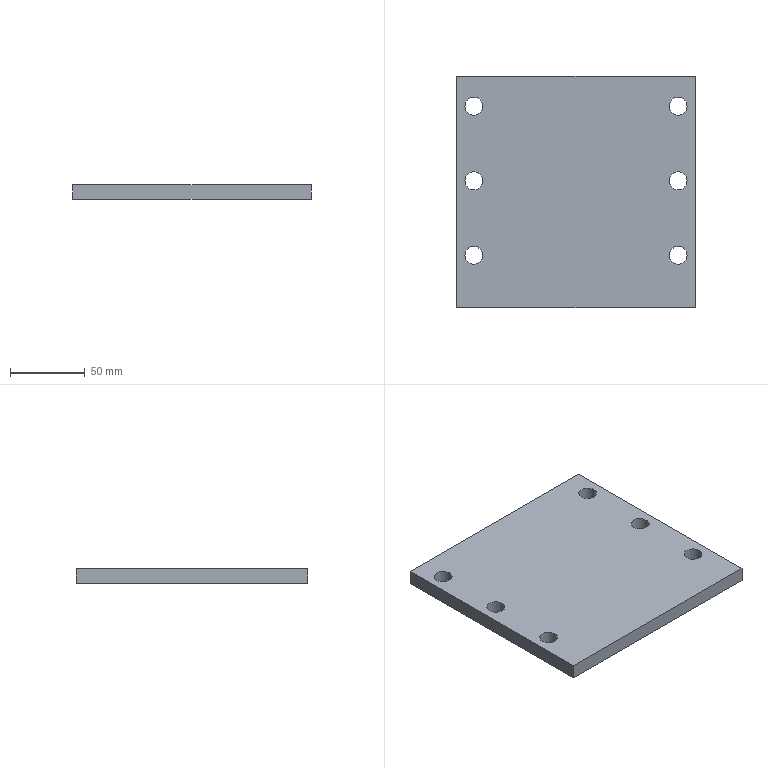Part | SolidWorks | features BaseBody 1 | 1 solid | 18 faces | box 160 x 155 x 10 mm | volume 241214 mm3 | cylinder 12 | plane 6 | commonest cylinder face diameters 12 x12
STEP:
#1=CARTESIAN_POINT('',(-0.01949,144.091,0.));
#2=VERTEX_POINT('',#1);
#3=CARTESIAN_POINT('',(-12.019,144.091,0.));
#4=VERTEX_POINT('',#3);
#5=CARTESIAN_POINT('',(-6.019,144.091,0.));
#6=DIRECTION('',(0.,0.,-1.));
#7=DIRECTION('',(1.,0.,0.));
#8=AXIS2_PLACEMENT_3D('',#5,#6,#7);
#9=CIRCLE('',#8,6.);
#10=EDGE_CURVE('',#2,#4,#9,.T.);
#11=ORIENTED_EDGE('',*,*,#10,.T.);
#12=CARTESIAN_POINT('',(-12.019,144.091,10.));
#13=VERTEX_POINT('',#12);
#14=CARTESIAN_POINT('',(-12.019,144.091,0.));
#15=DIRECTION('',(0.,0.,1.));
#16=VECTOR('',#15,1000.);
#17=LINE('',#14,#16);
#18=EDGE_CURVE('',#4,#13,#17,.T.);
#19=ORIENTED_EDGE('',*,*,#18,.T.);
#20=CARTESIAN_POINT('',(-0.01949,144.091,10.));
#21=VERTEX_POINT('',#20);
#22=CARTESIAN_POINT('',(-6.019,144.091,10.));
#23=DIRECTION('',(0.,0.,-1.));
#24=DIRECTION('',(1.,0.,0.));
#25=AXIS2_PLACEMENT_3D('',#22,#23,#24);
#26=CIRCLE('',#25,6.);
#27=EDGE_CURVE('',#21,#13,#26,.T.);
#28=ORIENTED_EDGE('',*,*,#27,.F.);
#29=CARTESIAN_POINT('',(-0.01949,144.091,0.));
#30=DIRECTION('',(0.,0.,1.));
#31=VECTOR('',#30,1000.);
#32=LINE('',#29,#31);
#33=EDGE_CURVE('',#2,#21,#32,.T.);
#34=ORIENTED_EDGE('',*,*,#33,.F.);
#35=EDGE_LOOP('',(#11,#19,#28,#34));
#36=FACE_OUTER_BOUND('',#35,.T.);
#37=CARTESIAN_POINT('',(-6.019,144.091,0.));
#38=DIRECTION('',(0.,0.,1.));
#39=DIRECTION('',(1.,0.,0.));
#40=AXIS2_PLACEMENT_3D('',#37,#38,#39);
#41=CYLINDRICAL_SURFACE('',#40,6.);
#42=ADVANCED_FACE('',(#36),#41,.F.);
#43=CARTESIAN_POINT('',(136.981,144.091,0.));
#44=VERTEX_POINT('',#43);
#45=CARTESIAN_POINT('',(124.981,144.091,0.));
#46=VERTEX_POINT('',#45);
#47=CARTESIAN_POINT('',(130.981,144.091,0.));
#48=DIRECTION('',(0.,0.,-1.));
#49=DIRECTION('',(1.,0.,0.));
#50=AXIS2_PLACEMENT_3D('',#47,#48,#49);
#51=CIRCLE('',#50,6.);
#52=EDGE_CURVE('',#44,#46,#51,.T.);
#53=ORIENTED_EDGE('',*,*,#52,.T.);
#54=CARTESIAN_POINT('',(124.981,144.091,10.));
#55=VERTEX_POINT('',#54);
#56=CARTESIAN_POINT('',(124.981,144.091,0.));
#57=DIRECTION('',(0.,0.,1.));
#58=VECTOR('',#57,1000.);
#59=LINE('',#56,#58);
#60=EDGE_CURVE('',#46,#55,#59,.T.);
#61=ORIENTED_EDGE('',*,*,#60,.T.);
#62=CARTESIAN_POINT('',(136.981,144.091,10.));
#63=VERTEX_POINT('',#62);
#64=CARTESIAN_POINT('',(130.981,144.091,10.));
#65=DIRECTION('',(0.,0.,-1.));
#66=DIRECTION('',(1.,0.,0.));
#67=AXIS2_PLACEMENT_3D('',#64,#65,#66);
#68=CIRCLE('',#67,6.);
#69=EDGE_CURVE('',#63,#55,#68,.T.);
#70=ORIENTED_EDGE('',*,*,#69,.F.);
#71=CARTESIAN_POINT('',(136.981,144.091,0.));
#72=DIRECTION('',(0.,0.,1.));
#73=VECTOR('',#72,1000.);
#74=LINE('',#71,#73);
#75=EDGE_CURVE('',#44,#63,#74,.T.);
#76=ORIENTED_EDGE('',*,*,#75,.F.);
#77=EDGE_LOOP('',(#53,#61,#70,#76));
#78=FACE_OUTER_BOUND('',#77,.T.);
#79=CARTESIAN_POINT('',(130.981,144.091,0.));
#80=DIRECTION('',(0.,0.,1.));
#81=DIRECTION('',(1.,0.,0.));
#82=AXIS2_PLACEMENT_3D('',#79,#80,#81);
#83=CYLINDRICAL_SURFACE('',#82,6.);
#84=ADVANCED_FACE('',(#78),#83,.F.);
#85=CARTESIAN_POINT('',(-0.01949,94.091,0.));
#86=VERTEX_POINT('',#85);
#87=CARTESIAN_POINT('',(-12.019,94.091,0.));
#88=VERTEX_POINT('',#87);
#89=CARTESIAN_POINT('',(-6.019,94.091,0.));
#90=DIRECTION('',(0.,0.,-1.));
#91=DIRECTION('',(1.,0.,0.));
#92=AXIS2_PLACEMENT_3D('',#89,#90,#91);
#93=CIRCLE('',#92,6.);
#94=EDGE_CURVE('',#86,#88,#93,.T.);
#95=ORIENTED_EDGE('',*,*,#94,.T.);
#96=CARTESIAN_POINT('',(-12.019,94.091,10.));
#97=VERTEX_POINT('',#96);
#98=CARTESIAN_POINT('',(-12.019,94.091,0.));
#99=DIRECTION('',(0.,0.,1.));
#100=VECTOR('',#99,1000.);
#101=LINE('',#98,#100);
#102=EDGE_CURVE('',#88,#97,#101,.T.);
#103=ORIENTED_EDGE('',*,*,#102,.T.);
#104=CARTESIAN_POINT('',(-0.01949,94.091,10.));
#105=VERTEX_POINT('',#104);
#106=CARTESIAN_POINT('',(-6.019,94.091,10.));
#107=DIRECTION('',(0.,0.,-1.));
#108=DIRECTION('',(1.,0.,0.));
#109=AXIS2_PLACEMENT_3D('',#106,#107,#108);
#110=CIRCLE('',#109,6.);
#111=EDGE_CURVE('',#105,#97,#110,.T.);
#112=ORIENTED_EDGE('',*,*,#111,.F.);
#113=CARTESIAN_POINT('',(-0.01949,94.091,0.));
#114=DIRECTION('',(0.,0.,1.));
#115=VECTOR('',#114,1000.);
#116=LINE('',#113,#115);
#117=EDGE_CURVE('',#86,#105,#116,.T.);
#118=ORIENTED_EDGE('',*,*,#117,.F.);
#119=EDGE_LOOP('',(#95,#103,#112,#118));
#120=FACE_OUTER_BOUND('',#119,.T.);
#121=CARTESIAN_POINT('',(-6.019,94.091,0.));
#122=DIRECTION('',(0.,0.,1.));
#123=DIRECTION('',(1.,0.,0.));
#124=AXIS2_PLACEMENT_3D('',#121,#122,#123);
#125=CYLINDRICAL_SURFACE('',#124,6.);
#126=ADVANCED_FACE('',(#120),#125,.F.);
#127=CARTESIAN_POINT('',(136.981,94.091,0.));
#128=VERTEX_POINT('',#127);
#129=CARTESIAN_POINT('',(124.981,94.091,0.));
#130=VERTEX_POINT('',#129);
#131=CARTESIAN_POINT('',(130.981,94.091,0.));
#132=DIRECTION('',(0.,0.,-1.));
#133=DIRECTION('',(1.,0.,0.));
#134=AXIS2_PLACEMENT_3D('',#131,#132,#133);
#135=CIRCLE('',#134,6.);
#136=EDGE_CURVE('',#128,#130,#135,.T.);
#137=ORIENTED_EDGE('',*,*,#136,.T.);
#138=CARTESIAN_POINT('',(124.981,94.091,10.));
#139=VERTEX_POINT('',#138);
#140=CARTESIAN_POINT('',(124.981,94.091,0.));
#141=DIRECTION('',(0.,0.,1.));
#142=VECTOR('',#141,1000.);
#143=LINE('',#140,#142);
#144=EDGE_CURVE('',#130,#139,#143,.T.);
#145=ORIENTED_EDGE('',*,*,#144,.T.);
#146=CARTESIAN_POINT('',(136.981,94.091,10.));
#147=VERTEX_POINT('',#146);
#148=CARTESIAN_POINT('',(130.981,94.091,10.));
#149=DIRECTION('',(0.,0.,-1.));
#150=DIRECTION('',(1.,0.,0.));
#151=AXIS2_PLACEMENT_3D('',#148,#149,#150);
#152=CIRCLE('',#151,6.);
#153=EDGE_CURVE('',#147,#139,#152,.T.);
#154=ORIENTED_EDGE('',*,*,#153,.F.);
#155=CARTESIAN_POINT('',(136.981,94.091,0.));
#156=DIRECTION('',(0.,0.,1.));
#157=VECTOR('',#156,1000.);
#158=LINE('',#155,#157);
#159=EDGE_CURVE('',#128,#147,#158,.T.);
#160=ORIENTED_EDGE('',*,*,#159,.F.);
#161=EDGE_LOOP('',(#137,#145,#154,#160));
#162=FACE_OUTER_BOUND('',#161,.T.);
#163=CARTESIAN_POINT('',(130.981,94.091,0.));
#164=DIRECTION('',(0.,0.,1.));
#165=DIRECTION('',(1.,0.,0.));
#166=AXIS2_PLACEMENT_3D('',#163,#164,#165);
#167=CYLINDRICAL_SURFACE('',#166,6.);
#168=ADVANCED_FACE('',(#162),#167,.F.);
#169=CARTESIAN_POINT('',(-0.01949,44.091,0.));
#170=VERTEX_POINT('',#169);
#171=CARTESIAN_POINT('',(-12.019,44.091,0.));
#172=VERTEX_POINT('',#171);
#173=CARTESIAN_POINT('',(-6.019,44.091,0.));
#174=DIRECTION('',(0.,0.,-1.));
#175=DIRECTION('',(1.,0.,0.));
#176=AXIS2_PLACEMENT_3D('',#173,#174,#175);
#177=CIRCLE('',#176,6.);
#178=EDGE_CURVE('',#170,#172,#177,.T.);
#179=ORIENTED_EDGE('',*,*,#178,.T.);
#180=CARTESIAN_POINT('',(-12.019,44.091,10.));
#181=VERTEX_POINT('',#180);
#182=CARTESIAN_POINT('',(-12.019,44.091,0.));
#183=DIRECTION('',(0.,0.,1.));
#184=VECTOR('',#183,1000.);
#185=LINE('',#182,#184);
#186=EDGE_CURVE('',#172,#181,#185,.T.);
#187=ORIENTED_EDGE('',*,*,#186,.T.);
#188=CARTESIAN_POINT('',(-0.01949,44.091,10.));
#189=VERTEX_POINT('',#188);
#190=CARTESIAN_POINT('',(-6.019,44.091,10.));
#191=DIRECTION('',(0.,0.,-1.));
#192=DIRECTION('',(1.,0.,0.));
#193=AXIS2_PLACEMENT_3D('',#190,#191,#192);
#194=CIRCLE('',#193,6.);
#195=EDGE_CURVE('',#189,#181,#194,.T.);
#196=ORIENTED_EDGE('',*,*,#195,.F.);
#197=CARTESIAN_POINT('',(-0.01949,44.091,0.));
#198=DIRECTION('',(0.,0.,1.));
#199=VECTOR('',#198,1000.);
#200=LINE('',#197,#199);
#201=EDGE_CURVE('',#170,#189,#200,.T.);
#202=ORIENTED_EDGE('',*,*,#201,.F.);
#203=EDGE_LOOP('',(#179,#187,#196,#202));
#204=FACE_OUTER_BOUND('',#203,.T.);
#205=CARTESIAN_POINT('',(-6.019,44.091,0.));
#206=DIRECTION('',(0.,0.,1.));
#207=DIRECTION('',(1.,0.,0.));
#208=AXIS2_PLACEMENT_3D('',#205,#206,#207);
#209=CYLINDRICAL_SURFACE('',#208,6.);
#210=ADVANCED_FACE('',(#204),#209,.F.);
#211=CARTESIAN_POINT('',(136.981,44.091,0.));
#212=VERTEX_POINT('',#211);
#213=CARTESIAN_POINT('',(124.981,44.091,0.));
#214=VERTEX_POINT('',#213);
#215=CARTESIAN_POINT('',(130.981,44.091,0.));
#216=DIRECTION('',(0.,0.,-1.));
#217=DIRECTION('',(1.,0.,0.));
#218=AXIS2_PLACEMENT_3D('',#215,#216,#217);
#219=CIRCLE('',#218,6.);
#220=EDGE_CURVE('',#212,#214,#219,.T.);
#221=ORIENTED_EDGE('',*,*,#220,.T.);
#222=CARTESIAN_POINT('',(124.981,44.091,10.));
#223=VERTEX_POINT('',#222);
#224=CARTESIAN_POINT('',(124.981,44.091,0.));
#225=DIRECTION('',(0.,0.,1.));
#226=VECTOR('',#225,1000.);
#227=LINE('',#224,#226);
#228=EDGE_CURVE('',#214,#223,#227,.T.);
#229=ORIENTED_EDGE('',*,*,#228,.T.);
#230=CARTESIAN_POINT('',(136.981,44.091,10.));
#231=VERTEX_POINT('',#230);
#232=CARTESIAN_POINT('',(130.981,44.091,10.));
#233=DIRECTION('',(0.,0.,-1.));
#234=DIRECTION('',(1.,0.,0.));
#235=AXIS2_PLACEMENT_3D('',#232,#233,#234);
#236=CIRCLE('',#235,6.);
#237=EDGE_CURVE('',#231,#223,#236,.T.);
#238=ORIENTED_EDGE('',*,*,#237,.F.);
#239=CARTESIAN_POINT('',(136.981,44.091,0.));
#240=DIRECTION('',(0.,0.,1.));
#241=VECTOR('',#240,1000.);
#242=LINE('',#239,#241);
#243=EDGE_CURVE('',#212,#231,#242,.T.);
#244=ORIENTED_EDGE('',*,*,#243,.F.);
#245=EDGE_LOOP('',(#221,#229,#238,#244));
#246=FACE_OUTER_BOUND('',#245,.T.);
#247=CARTESIAN_POINT('',(130.981,44.091,0.));
#248=DIRECTION('',(0.,0.,1.));
#249=DIRECTION('',(1.,0.,0.));
#250=AXIS2_PLACEMENT_3D('',#247,#248,#249);
#251=CYLINDRICAL_SURFACE('',#250,6.);
#252=ADVANCED_FACE('',(#246),#251,.F.);
#253=ORIENTED_EDGE('',*,*,#10,.F.);
#254=CARTESIAN_POINT('',(-6.019,144.091,0.));
#255=DIRECTION('',(0.,0.,-1.));
#256=DIRECTION('',(1.,0.,0.));
#257=AXIS2_PLACEMENT_3D('',#254,#255,#256);
#258=CIRCLE('',#257,6.);
#259=EDGE_CURVE('',#4,#2,#258,.T.);
#260=ORIENTED_EDGE('',*,*,#259,.F.);
#261=EDGE_LOOP('',(#253,#260));
#262=FACE_BOUND('',#261,.T.);
#263=ORIENTED_EDGE('',*,*,#52,.F.);
#264=CARTESIAN_POINT('',(130.981,144.091,0.));
#265=DIRECTION('',(0.,0.,-1.));
#266=DIRECTION('',(1.,0.,0.));
#267=AXIS2_PLACEMENT_3D('',#264,#265,#266);
#268=CIRCLE('',#267,6.);
#269=EDGE_CURVE('',#46,#44,#268,.T.);
#270=ORIENTED_EDGE('',*,*,#269,.F.);
#271=EDGE_LOOP('',(#263,#270));
#272=FACE_BOUND('',#271,.T.);
#273=ORIENTED_EDGE('',*,*,#94,.F.);
#274=CARTESIAN_POINT('',(-6.019,94.091,0.));
#275=DIRECTION('',(0.,0.,-1.));
#276=DIRECTION('',(1.,0.,0.));
#277=AXIS2_PLACEMENT_3D('',#274,#275,#276);
#278=CIRCLE('',#277,6.);
#279=EDGE_CURVE('',#88,#86,#278,.T.);
#280=ORIENTED_EDGE('',*,*,#279,.F.);
#281=EDGE_LOOP('',(#273,#280));
#282=FACE_BOUND('',#281,.T.);
#283=ORIENTED_EDGE('',*,*,#136,.F.);
#284=CARTESIAN_POINT('',(130.981,94.091,0.));
#285=DIRECTION('',(0.,0.,-1.));
#286=DIRECTION('',(1.,0.,0.));
#287=AXIS2_PLACEMENT_3D('',#284,#285,#286);
#288=CIRCLE('',#287,6.);
#289=EDGE_CURVE('',#130,#128,#288,.T.);
#290=ORIENTED_EDGE('',*,*,#289,.F.);
#291=EDGE_LOOP('',(#283,#290));
#292=FACE_BOUND('',#291,.T.);
#293=ORIENTED_EDGE('',*,*,#178,.F.);
#294=CARTESIAN_POINT('',(-6.019,44.091,0.));
#295=DIRECTION('',(0.,0.,-1.));
#296=DIRECTION('',(1.,0.,0.));
#297=AXIS2_PLACEMENT_3D('',#294,#295,#296);
#298=CIRCLE('',#297,6.);
#299=EDGE_CURVE('',#172,#170,#298,.T.);
#300=ORIENTED_EDGE('',*,*,#299,.F.);
#301=EDGE_LOOP('',(#293,#300));
#302=FACE_BOUND('',#301,.T.);
#303=ORIENTED_EDGE('',*,*,#220,.F.);
#304=CARTESIAN_POINT('',(130.981,44.091,0.));
#305=DIRECTION('',(0.,0.,-1.));
#306=DIRECTION('',(1.,0.,0.));
#307=AXIS2_PLACEMENT_3D('',#304,#305,#306);
#308=CIRCLE('',#307,6.);
#309=EDGE_CURVE('',#214,#212,#308,.T.);
#310=ORIENTED_EDGE('',*,*,#309,.F.);
#311=EDGE_LOOP('',(#303,#310));
#312=FACE_BOUND('',#311,.T.);
#313=CARTESIAN_POINT('',(142.481,164.091,0.));
#314=VERTEX_POINT('',#313);
#315=CARTESIAN_POINT('',(-17.519,164.091,0.));
#316=VERTEX_POINT('',#315);
#317=CARTESIAN_POINT('',(62.481,164.091,0.));
#318=DIRECTION('',(-1.,0.,0.));
#319=VECTOR('',#318,1000.);
#320=LINE('',#317,#319);
#321=EDGE_CURVE('',#314,#316,#320,.T.);
#322=ORIENTED_EDGE('',*,*,#321,.F.);
#323=CARTESIAN_POINT('',(142.481,9.091,0.));
#324=VERTEX_POINT('',#323);
#325=CARTESIAN_POINT('',(142.481,86.591,0.));
#326=DIRECTION('',(0.,1.,0.));
#327=VECTOR('',#326,1000.);
#328=LINE('',#325,#327);
#329=EDGE_CURVE('',#324,#314,#328,.T.);
#330=ORIENTED_EDGE('',*,*,#329,.F.);
#331=CARTESIAN_POINT('',(-17.519,9.091,0.));
#332=VERTEX_POINT('',#331);
#333=CARTESIAN_POINT('',(62.481,9.091,0.));
#334=DIRECTION('',(1.,0.,0.));
#335=VECTOR('',#334,1000.);
#336=LINE('',#333,#335);
#337=EDGE_CURVE('',#332,#324,#336,.T.);
#338=ORIENTED_EDGE('',*,*,#337,.F.);
#339=CARTESIAN_POINT('',(-17.519,86.591,0.));
#340=DIRECTION('',(0.,-1.,0.));
#341=VECTOR('',#340,1000.);
#342=LINE('',#339,#341);
#343=EDGE_CURVE('',#316,#332,#342,.T.);
#344=ORIENTED_EDGE('',*,*,#343,.F.);
#345=EDGE_LOOP('',(#322,#330,#338,#344));
#346=FACE_OUTER_BOUND('',#345,.T.);
#347=CARTESIAN_POINT('',(62.481,86.591,0.));
#348=DIRECTION('',(0.,0.,1.));
#349=DIRECTION('',(1.,0.,0.));
#350=AXIS2_PLACEMENT_3D('',#347,#348,#349);
#351=PLANE('',#350);
#352=ADVANCED_FACE('',(#262,#272,#282,#292,#302,#312,#346),#351,.F.);
#353=ORIENTED_EDGE('',*,*,#18,.F.);
#354=ORIENTED_EDGE('',*,*,#259,.T.);
#355=ORIENTED_EDGE('',*,*,#33,.T.);
#356=CARTESIAN_POINT('',(-6.019,144.091,10.));
#357=DIRECTION('',(0.,0.,-1.));
#358=DIRECTION('',(1.,0.,0.));
#359=AXIS2_PLACEMENT_3D('',#356,#357,#358);
#360=CIRCLE('',#359,6.);
#361=EDGE_CURVE('',#13,#21,#360,.T.);
#362=ORIENTED_EDGE('',*,*,#361,.F.);
#363=EDGE_LOOP('',(#353,#354,#355,#362));
#364=FACE_OUTER_BOUND('',#363,.T.);
#365=CARTESIAN_POINT('',(-6.019,144.091,0.));
#366=DIRECTION('',(0.,0.,1.));
#367=DIRECTION('',(1.,0.,0.));
#368=AXIS2_PLACEMENT_3D('',#365,#366,#367);
#369=CYLINDRICAL_SURFACE('',#368,6.);
#370=ADVANCED_FACE('',(#364),#369,.F.);
#371=ORIENTED_EDGE('',*,*,#60,.F.);
#372=ORIENTED_EDGE('',*,*,#269,.T.);
#373=ORIENTED_EDGE('',*,*,#75,.T.);
#374=CARTESIAN_POINT('',(130.981,144.091,10.));
#375=DIRECTION('',(0.,0.,-1.));
#376=DIRECTION('',(1.,0.,0.));
#377=AXIS2_PLACEMENT_3D('',#374,#375,#376);
#378=CIRCLE('',#377,6.);
#379=EDGE_CURVE('',#55,#63,#378,.T.);
#380=ORIENTED_EDGE('',*,*,#379,.F.);
#381=EDGE_LOOP('',(#371,#372,#373,#380));
#382=FACE_OUTER_BOUND('',#381,.T.);
#383=CARTESIAN_POINT('',(130.981,144.091,0.));
#384=DIRECTION('',(0.,0.,1.));
#385=DIRECTION('',(1.,0.,0.));
#386=AXIS2_PLACEMENT_3D('',#383,#384,#385);
#387=CYLINDRICAL_SURFACE('',#386,6.);
#388=ADVANCED_FACE('',(#382),#387,.F.);
#389=ORIENTED_EDGE('',*,*,#102,.F.);
#390=ORIENTED_EDGE('',*,*,#279,.T.);
#391=ORIENTED_EDGE('',*,*,#117,.T.);
#392=CARTESIAN_POINT('',(-6.019,94.091,10.));
#393=DIRECTION('',(0.,0.,-1.));
#394=DIRECTION('',(1.,0.,0.));
#395=AXIS2_PLACEMENT_3D('',#392,#393,#394);
#396=CIRCLE('',#395,6.);
#397=EDGE_CURVE('',#97,#105,#396,.T.);
#398=ORIENTED_EDGE('',*,*,#397,.F.);
#399=EDGE_LOOP('',(#389,#390,#391,#398));
#400=FACE_OUTER_BOUND('',#399,.T.);
#401=CARTESIAN_POINT('',(-6.019,94.091,0.));
#402=DIRECTION('',(0.,0.,1.));
#403=DIRECTION('',(1.,0.,0.));
#404=AXIS2_PLACEMENT_3D('',#401,#402,#403);
#405=CYLINDRICAL_SURFACE('',#404,6.);
#406=ADVANCED_FACE('',(#400),#405,.F.);
#407=ORIENTED_EDGE('',*,*,#144,.F.);
#408=ORIENTED_EDGE('',*,*,#289,.T.);
#409=ORIENTED_EDGE('',*,*,#159,.T.);
#410=CARTESIAN_POINT('',(130.981,94.091,10.));
#411=DIRECTION('',(0.,0.,-1.));
#412=DIRECTION('',(1.,0.,0.));
#413=AXIS2_PLACEMENT_3D('',#410,#411,#412);
#414=CIRCLE('',#413,6.);
#415=EDGE_CURVE('',#139,#147,#414,.T.);
#416=ORIENTED_EDGE('',*,*,#415,.F.);
#417=EDGE_LOOP('',(#407,#408,#409,#416));
#418=FACE_OUTER_BOUND('',#417,.T.);
#419=CARTESIAN_POINT('',(130.981,94.091,0.));
#420=DIRECTION('',(0.,0.,1.));
#421=DIRECTION('',(1.,0.,0.));
#422=AXIS2_PLACEMENT_3D('',#419,#420,#421);
#423=CYLINDRICAL_SURFACE('',#422,6.);
#424=ADVANCED_FACE('',(#418),#423,.F.);
#425=ORIENTED_EDGE('',*,*,#186,.F.);
#426=ORIENTED_EDGE('',*,*,#299,.T.);
#427=ORIENTED_EDGE('',*,*,#201,.T.);
#428=CARTESIAN_POINT('',(-6.019,44.091,10.));
#429=DIRECTION('',(0.,0.,-1.));
#430=DIRECTION('',(1.,0.,0.));
#431=AXIS2_PLACEMENT_3D('',#428,#429,#430);
#432=CIRCLE('',#431,6.);
#433=EDGE_CURVE('',#181,#189,#432,.T.);
#434=ORIENTED_EDGE('',*,*,#433,.F.);
#435=EDGE_LOOP('',(#425,#426,#427,#434));
#436=FACE_OUTER_BOUND('',#435,.T.);
#437=CARTESIAN_POINT('',(-6.019,44.091,0.));
#438=DIRECTION('',(0.,0.,1.));
#439=DIRECTION('',(1.,0.,0.));
#440=AXIS2_PLACEMENT_3D('',#437,#438,#439);
#441=CYLINDRICAL_SURFACE('',#440,6.);
#442=ADVANCED_FACE('',(#436),#441,.F.);
#443=ORIENTED_EDGE('',*,*,#228,.F.);
#444=ORIENTED_EDGE('',*,*,#309,.T.);
#445=ORIENTED_EDGE('',*,*,#243,.T.);
#446=CARTESIAN_POINT('',(130.981,44.091,10.));
#447=DIRECTION('',(0.,0.,-1.));
#448=DIRECTION('',(1.,0.,0.));
#449=AXIS2_PLACEMENT_3D('',#446,#447,#448);
#450=CIRCLE('',#449,6.);
#451=EDGE_CURVE('',#223,#231,#450,.T.);
#452=ORIENTED_EDGE('',*,*,#451,.F.);
#453=EDGE_LOOP('',(#443,#444,#445,#452));
#454=FACE_OUTER_BOUND('',#453,.T.);
#455=CARTESIAN_POINT('',(130.981,44.091,0.));
#456=DIRECTION('',(0.,0.,1.));
#457=DIRECTION('',(1.,0.,0.));
#458=AXIS2_PLACEMENT_3D('',#455,#456,#457);
#459=CYLINDRICAL_SURFACE('',#458,6.);
#460=ADVANCED_FACE('',(#454),#459,.F.);
#461=ORIENTED_EDGE('',*,*,#343,.T.);
#462=CARTESIAN_POINT('',(-17.519,9.091,10.));
#463=VERTEX_POINT('',#462);
#464=CARTESIAN_POINT('',(-17.519,9.091,0.));
#465=DIRECTION('',(0.,0.,1.));
#466=VECTOR('',#465,1000.);
#467=LINE('',#464,#466);
#468=EDGE_CURVE('',#332,#463,#467,.T.);
#469=ORIENTED_EDGE('',*,*,#468,.T.);
#470=CARTESIAN_POINT('',(-17.519,164.091,10.));
#471=VERTEX_POINT('',#470);
#472=CARTESIAN_POINT('',(-17.519,9.091,10.));
#473=DIRECTION('',(0.,1.,0.));
#474=VECTOR('',#473,1000.);
#475=LINE('',#472,#474);
#476=EDGE_CURVE('',#463,#471,#475,.T.);
#477=ORIENTED_EDGE('',*,*,#476,.T.);
#478=CARTESIAN_POINT('',(-17.519,164.091,0.));
#479=DIRECTION('',(0.,0.,-1.));
#480=VECTOR('',#479,1000.);
#481=LINE('',#478,#480);
#482=EDGE_CURVE('',#471,#316,#481,.T.);
#483=ORIENTED_EDGE('',*,*,#482,.T.);
#484=EDGE_LOOP('',(#461,#469,#477,#483));
#485=FACE_OUTER_BOUND('',#484,.T.);
#486=CARTESIAN_POINT('',(-17.519,9.091,0.));
#487=DIRECTION('',(-1.,0.,0.));
#488=DIRECTION('',(0.,-1.,0.));
#489=AXIS2_PLACEMENT_3D('',#486,#487,#488);
#490=PLANE('',#489);
#491=ADVANCED_FACE('',(#485),#490,.T.);
#492=ORIENTED_EDGE('',*,*,#321,.T.);
#493=ORIENTED_EDGE('',*,*,#482,.F.);
#494=CARTESIAN_POINT('',(142.481,164.091,10.));
#495=VERTEX_POINT('',#494);
#496=CARTESIAN_POINT('',(-17.519,164.091,10.));
#497=DIRECTION('',(1.,0.,0.));
#498=VECTOR('',#497,1000.);
#499=LINE('',#496,#498);
#500=EDGE_CURVE('',#471,#495,#499,.T.);
#501=ORIENTED_EDGE('',*,*,#500,.T.);
#502=CARTESIAN_POINT('',(142.481,164.091,0.));
#503=DIRECTION('',(0.,0.,-1.));
#504=VECTOR('',#503,1000.);
#505=LINE('',#502,#504);
#506=EDGE_CURVE('',#495,#314,#505,.T.);
#507=ORIENTED_EDGE('',*,*,#506,.T.);
#508=EDGE_LOOP('',(#492,#493,#501,#507));
#509=FACE_OUTER_BOUND('',#508,.T.);
#510=CARTESIAN_POINT('',(-17.519,164.091,0.));
#511=DIRECTION('',(0.,1.,0.));
#512=DIRECTION('',(0.,0.,1.));
#513=AXIS2_PLACEMENT_3D('',#510,#511,#512);
#514=PLANE('',#513);
#515=ADVANCED_FACE('',(#509),#514,.T.);
#516=ORIENTED_EDGE('',*,*,#329,.T.);
#517=ORIENTED_EDGE('',*,*,#506,.F.);
#518=CARTESIAN_POINT('',(142.481,9.091,10.));
#519=VERTEX_POINT('',#518);
#520=CARTESIAN_POINT('',(142.481,164.091,10.));
#521=DIRECTION('',(0.,-1.,0.));
#522=VECTOR('',#521,1000.);
#523=LINE('',#520,#522);
#524=EDGE_CURVE('',#495,#519,#523,.T.);
#525=ORIENTED_EDGE('',*,*,#524,.T.);
#526=CARTESIAN_POINT('',(142.481,9.091,0.));
#527=DIRECTION('',(0.,0.,-1.));
#528=VECTOR('',#527,1000.);
#529=LINE('',#526,#528);
#530=EDGE_CURVE('',#519,#324,#529,.T.);
#531=ORIENTED_EDGE('',*,*,#530,.T.);
#532=EDGE_LOOP('',(#516,#517,#525,#531));
#533=FACE_OUTER_BOUND('',#532,.T.);
#534=CARTESIAN_POINT('',(142.481,164.091,0.));
#535=DIRECTION('',(1.,0.,0.));
#536=DIRECTION('',(0.,0.,-1.));
#537=AXIS2_PLACEMENT_3D('',#534,#535,#536);
#538=PLANE('',#537);
#539=ADVANCED_FACE('',(#533),#538,.T.);
#540=ORIENTED_EDGE('',*,*,#337,.T.);
#541=ORIENTED_EDGE('',*,*,#530,.F.);
#542=CARTESIAN_POINT('',(142.481,9.091,10.));
#543=DIRECTION('',(-1.,0.,0.));
#544=VECTOR('',#543,1000.);
#545=LINE('',#542,#544);
#546=EDGE_CURVE('',#519,#463,#545,.T.);
#547=ORIENTED_EDGE('',*,*,#546,.T.);
#548=ORIENTED_EDGE('',*,*,#468,.F.);
#549=EDGE_LOOP('',(#540,#541,#547,#548));
#550=FACE_OUTER_BOUND('',#549,.T.);
#551=CARTESIAN_POINT('',(142.481,9.091,0.));
#552=DIRECTION('',(0.,-1.,0.));
#553=DIRECTION('',(1.,0.,0.));
#554=AXIS2_PLACEMENT_3D('',#551,#552,#553);
#555=PLANE('',#554);
#556=ADVANCED_FACE('',(#550),#555,.T.);
#557=ORIENTED_EDGE('',*,*,#27,.T.);
#558=ORIENTED_EDGE('',*,*,#361,.T.);
#559=EDGE_LOOP('',(#557,#558));
#560=FACE_BOUND('',#559,.T.);
#561=ORIENTED_EDGE('',*,*,#69,.T.);
#562=ORIENTED_EDGE('',*,*,#379,.T.);
#563=EDGE_LOOP('',(#561,#562));
#564=FACE_BOUND('',#563,.T.);
#565=ORIENTED_EDGE('',*,*,#111,.T.);
#566=ORIENTED_EDGE('',*,*,#397,.T.);
#567=EDGE_LOOP('',(#565,#566));
#568=FACE_BOUND('',#567,.T.);
#569=ORIENTED_EDGE('',*,*,#153,.T.);
#570=ORIENTED_EDGE('',*,*,#415,.T.);
#571=EDGE_LOOP('',(#569,#570));
#572=FACE_BOUND('',#571,.T.);
#573=ORIENTED_EDGE('',*,*,#195,.T.);
#574=ORIENTED_EDGE('',*,*,#433,.T.);
#575=EDGE_LOOP('',(#573,#574));
#576=FACE_BOUND('',#575,.T.);
#577=ORIENTED_EDGE('',*,*,#237,.T.);
#578=ORIENTED_EDGE('',*,*,#451,.T.);
#579=EDGE_LOOP('',(#577,#578));
#580=FACE_BOUND('',#579,.T.);
#581=ORIENTED_EDGE('',*,*,#546,.F.);
#582=ORIENTED_EDGE('',*,*,#524,.F.);
#583=ORIENTED_EDGE('',*,*,#500,.F.);
#584=ORIENTED_EDGE('',*,*,#476,.F.);
#585=EDGE_LOOP('',(#581,#582,#583,#584));
#586=FACE_OUTER_BOUND('',#585,.T.);
#587=CARTESIAN_POINT('',(62.481,86.591,10.));
#588=DIRECTION('',(0.,0.,1.));
#589=DIRECTION('',(1.,0.,0.));
#590=AXIS2_PLACEMENT_3D('',#587,#588,#589);
#591=PLANE('',#590);
#592=ADVANCED_FACE('',(#560,#564,#568,#572,#576,#580,#586),#591,.T.);
#593=CLOSED_SHELL('',(#42,#84,#126,#168,#210,#252,#352,#370,#388,#406,#424,#442,#460,#491,#515,#539,#556,#592));
#594=MANIFOLD_SOLID_BREP('',#593);
#595=CARTESIAN_POINT('',(0.,0.,0.));
#596=DIRECTION('',(0.,0.,1.));
#597=DIRECTION('',(1.,0.,0.));
#598=AXIS2_PLACEMENT_3D('',#595,#596,#597);
#599=(LENGTH_UNIT()NAMED_UNIT(*)SI_UNIT(.MILLI.,.METRE.));
#600=UNCERTAINTY_MEASURE_WITH_UNIT(LENGTH_MEASURE(0.00001),#599,'','');
#601=(NAMED_UNIT(*)PLANE_ANGLE_UNIT()SI_UNIT($,.RADIAN.));
#602=(NAMED_UNIT(*)SI_UNIT($,.STERADIAN.)SOLID_ANGLE_UNIT());
#603=(GEOMETRIC_REPRESENTATION_CONTEXT(3)GLOBAL_UNCERTAINTY_ASSIGNED_CONTEXT((#600))GLOBAL_UNIT_ASSIGNED_CONTEXT((#599,#601,#602))REPRESENTATION_CONTEXT('',''));
#604=ADVANCED_BREP_SHAPE_REPRESENTATION('',(#594,#598),#603);